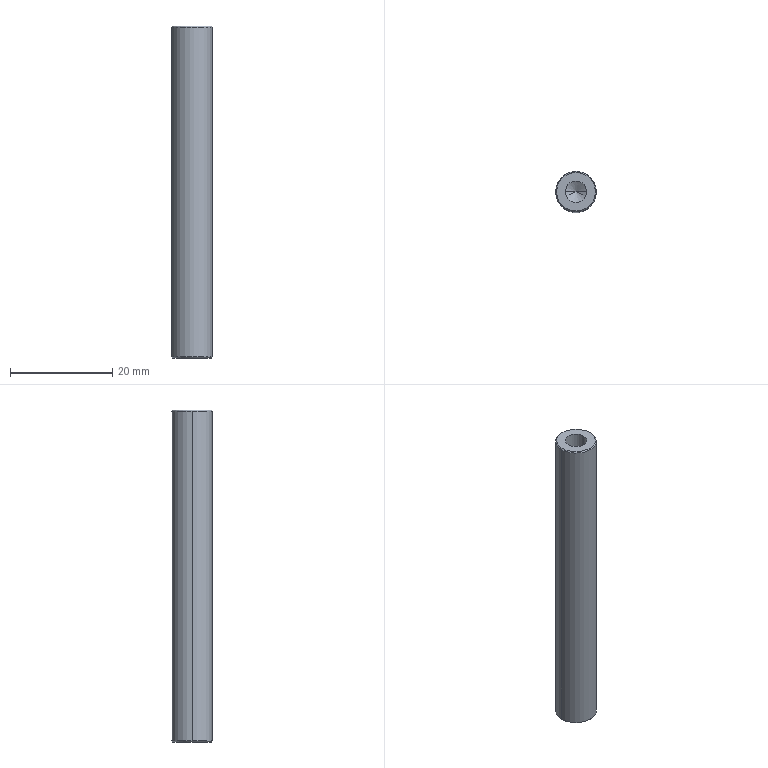Part | STEP file | 1 solid | 16 faces | box 8 x 8 x 65 mm | volume 2978 mm3 | cone 8 | cylinder 6 | plane 2 | commonest cylinder face diameters 4.2 x4 8 x2
STEP:
#1=CARTESIAN_POINT('',(0.,0.,0.));
#2=DIRECTION('',(0.,0.,1.));
#3=DIRECTION('',(1.,0.,0.));
#4=AXIS2_PLACEMENT_3D('',#1,#2,#3);
#5=CARTESIAN_POINT('',(-2.1,0.,-22.5));
#6=VERTEX_POINT('',#5);
#7=CARTESIAN_POINT('',(-2.1,0.,-32.5));
#8=VERTEX_POINT('',#7);
#9=CARTESIAN_POINT('',(-2.1,0.,-32.5));
#10=DIRECTION('',(0.,0.,-1.));
#11=VECTOR('',#10,1.);
#12=LINE('',#9,#11);
#13=CARTESIAN_POINT('',(0.,0.,-32.5));
#14=DIRECTION('',(0.,0.,-1.));
#15=DIRECTION('',(-1.,0.,0.));
#16=AXIS2_PLACEMENT_3D('',#13,#14,#15);
#17=CYLINDRICAL_SURFACE('',#16,2.1);
#18=CARTESIAN_POINT('',(6.283,0.));
#19=DIRECTION('',(0.,1.));
#20=VECTOR('',#19,1.);
#21=LINE('',#18,#20);
#22=(GEOMETRIC_REPRESENTATION_CONTEXT(2)PARAMETRIC_REPRESENTATION_CONTEXT()REPRESENTATION_CONTEXT('',''));
#23=DEFINITIONAL_REPRESENTATION('',(#21),#22);
#24=PCURVE('',#17,#23);
#25=CARTESIAN_POINT('',(0.,0.,-32.5));
#26=DIRECTION('',(0.,0.,-1.));
#27=DIRECTION('',(-1.,0.,0.));
#28=AXIS2_PLACEMENT_3D('',#25,#26,#27);
#29=CYLINDRICAL_SURFACE('',#28,2.1);
#30=CARTESIAN_POINT('',(0.,0.));
#31=DIRECTION('',(0.,1.));
#32=VECTOR('',#31,1.);
#33=LINE('',#30,#32);
#34=(GEOMETRIC_REPRESENTATION_CONTEXT(2)PARAMETRIC_REPRESENTATION_CONTEXT()REPRESENTATION_CONTEXT('',''));
#35=DEFINITIONAL_REPRESENTATION('',(#33),#34);
#36=PCURVE('',#29,#35);
#37=SURFACE_CURVE('',#12,(#24,#36),.PCURVE_S1.);
#38=EDGE_CURVE('',#6,#8,#37,.T.);
#39=ORIENTED_EDGE('',*,*,#38,.T.);
#40=CARTESIAN_POINT('',(2.1,0.,-32.5));
#41=VERTEX_POINT('',#40);
#42=CARTESIAN_POINT('',(0.,0.,-32.5));
#43=DIRECTION('',(0.,0.,-1.));
#44=DIRECTION('',(-1.,0.,0.));
#45=AXIS2_PLACEMENT_3D('',#42,#43,#44);
#46=CIRCLE('',#45,2.1);
#47=CARTESIAN_POINT('',(0.,0.));
#48=DIRECTION('',(1.,0.));
#49=VECTOR('',#48,1.);
#50=LINE('',#47,#49);
#51=(GEOMETRIC_REPRESENTATION_CONTEXT(2)PARAMETRIC_REPRESENTATION_CONTEXT()REPRESENTATION_CONTEXT('',''));
#52=DEFINITIONAL_REPRESENTATION('',(#50),#51);
#53=PCURVE('',#17,#52);
#54=CARTESIAN_POINT('',(0.,0.,-32.5));
#55=DIRECTION('',(0.,0.,1.));
#56=DIRECTION('',(1.,0.,0.));
#57=AXIS2_PLACEMENT_3D('',#54,#55,#56);
#58=PLANE('',#57);
#59=CARTESIAN_POINT('',(-2.1,0.));
#60=CARTESIAN_POINT('',(-2.1,3.637));
#61=CARTESIAN_POINT('',(1.05,1.819));
#62=CARTESIAN_POINT('',(4.2,0.));
#63=CARTESIAN_POINT('',(1.05,-1.819));
#64=CARTESIAN_POINT('',(-2.1,-3.637));
#65=CARTESIAN_POINT('',(-2.1,0.));
#66=(BOUNDED_CURVE()B_SPLINE_CURVE(2,(#59,#60,#61,#62,#63,#64,#65),.UNSPECIFIED.,.T.,.F.)B_SPLINE_CURVE_WITH_KNOTS((1,2,2,2,2,1),(-2.094,0.,2.094,4.189,6.283,8.378),.UNSPECIFIED.)CURVE()GEOMETRIC_REPRESENTATION_ITEM()RATIONAL_B_SPLINE_CURVE((1.,0.5,1.,0.5,1.,0.5,1.))REPRESENTATION_ITEM(''));
#67=(GEOMETRIC_REPRESENTATION_CONTEXT(2)PARAMETRIC_REPRESENTATION_CONTEXT()REPRESENTATION_CONTEXT('',''));
#68=DEFINITIONAL_REPRESENTATION('',(#66),#67);
#69=PCURVE('',#58,#68);
#70=SURFACE_CURVE('',#46,(#53,#69),.PCURVE_S1.);
#71=EDGE_CURVE('',#41,#8,#70,.T.);
#72=ORIENTED_EDGE('',*,*,#71,.F.);
#73=CARTESIAN_POINT('',(2.1,0.,-22.5));
#74=VERTEX_POINT('',#73);
#75=CARTESIAN_POINT('',(2.1,0.,-32.5));
#76=DIRECTION('',(0.,0.,-1.));
#77=VECTOR('',#76,1.);
#78=LINE('',#75,#77);
#79=CARTESIAN_POINT('',(3.142,0.));
#80=DIRECTION('',(0.,1.));
#81=VECTOR('',#80,1.);
#82=LINE('',#79,#81);
#83=(GEOMETRIC_REPRESENTATION_CONTEXT(2)PARAMETRIC_REPRESENTATION_CONTEXT()REPRESENTATION_CONTEXT('',''));
#84=DEFINITIONAL_REPRESENTATION('',(#82),#83);
#85=PCURVE('',#17,#84);
#86=CARTESIAN_POINT('',(3.142,0.));
#87=DIRECTION('',(0.,1.));
#88=VECTOR('',#87,1.);
#89=LINE('',#86,#88);
#90=(GEOMETRIC_REPRESENTATION_CONTEXT(2)PARAMETRIC_REPRESENTATION_CONTEXT()REPRESENTATION_CONTEXT('',''));
#91=DEFINITIONAL_REPRESENTATION('',(#89),#90);
#92=PCURVE('',#29,#91);
#93=SURFACE_CURVE('',#78,(#85,#92),.PCURVE_S1.);
#94=EDGE_CURVE('',#74,#41,#93,.T.);
#95=ORIENTED_EDGE('',*,*,#94,.F.);
#96=CARTESIAN_POINT('',(0.,0.,-22.5));
#97=DIRECTION('',(0.,0.,-1.));
#98=DIRECTION('',(-1.,0.,0.));
#99=AXIS2_PLACEMENT_3D('',#96,#97,#98);
#100=CIRCLE('',#99,2.1);
#101=CARTESIAN_POINT('',(0.,-10.));
#102=DIRECTION('',(1.,0.));
#103=VECTOR('',#102,1.);
#104=LINE('',#101,#103);
#105=(GEOMETRIC_REPRESENTATION_CONTEXT(2)PARAMETRIC_REPRESENTATION_CONTEXT()REPRESENTATION_CONTEXT('',''));
#106=DEFINITIONAL_REPRESENTATION('',(#104),#105);
#107=PCURVE('',#17,#106);
#108=CARTESIAN_POINT('',(0.,0.,-22.5));
#109=DIRECTION('',(0.,0.,-1.));
#110=DIRECTION('',(-1.,0.,0.));
#111=AXIS2_PLACEMENT_3D('',#108,#109,#110);
#112=CONICAL_SURFACE('',#111,2.1,1.03);
#113=CARTESIAN_POINT('',(0.,0.));
#114=DIRECTION('',(1.,0.));
#115=VECTOR('',#114,1.);
#116=LINE('',#113,#115);
#117=(GEOMETRIC_REPRESENTATION_CONTEXT(2)PARAMETRIC_REPRESENTATION_CONTEXT()REPRESENTATION_CONTEXT('',''));
#118=DEFINITIONAL_REPRESENTATION('',(#116),#117);
#119=PCURVE('',#112,#118);
#120=SURFACE_CURVE('',#100,(#107,#119),.PCURVE_S1.);
#121=EDGE_CURVE('',#74,#6,#120,.T.);
#122=ORIENTED_EDGE('',*,*,#121,.T.);
#123=EDGE_LOOP('',(#39,#72,#95,#122));
#124=FACE_BOUND('',#123,.F.);
#125=ADVANCED_FACE('',(#124),#17,.F.);
#126=ORIENTED_EDGE('',*,*,#121,.F.);
#127=CARTESIAN_POINT('',(0.,0.,-21.238));
#128=VERTEX_POINT('',#127);
#129=CARTESIAN_POINT('',(2.1,0.,-22.5));
#130=DIRECTION('',(0.8572,0.,-0.515));
#131=VECTOR('',#130,1.);
#132=LINE('',#129,#131);
#133=CARTESIAN_POINT('',(3.142,-1.262));
#134=CARTESIAN_POINT('',(3.142,-1.243));
#135=CARTESIAN_POINT('',(3.142,-1.204));
#136=CARTESIAN_POINT('',(3.142,-1.147));
#137=CARTESIAN_POINT('',(3.142,-1.09));
#138=CARTESIAN_POINT('',(3.142,-1.032));
#139=CARTESIAN_POINT('',(3.142,-0.975));
#140=CARTESIAN_POINT('',(3.142,-0.9177));
#141=CARTESIAN_POINT('',(3.142,-0.8603));
#142=CARTESIAN_POINT('',(3.142,-0.803));
#143=CARTESIAN_POINT('',(3.142,-0.7456));
#144=CARTESIAN_POINT('',(3.142,-0.6883));
#145=CARTESIAN_POINT('',(3.142,-0.6309));
#146=CARTESIAN_POINT('',(3.142,-0.5735));
#147=CARTESIAN_POINT('',(3.142,-0.5162));
#148=CARTESIAN_POINT('',(3.142,-0.4588));
#149=CARTESIAN_POINT('',(3.142,-0.4015));
#150=CARTESIAN_POINT('',(3.142,-0.3441));
#151=CARTESIAN_POINT('',(3.142,-0.2868));
#152=CARTESIAN_POINT('',(3.142,-0.2294));
#153=CARTESIAN_POINT('',(3.142,-0.1721));
#154=CARTESIAN_POINT('',(3.142,-0.1147));
#155=CARTESIAN_POINT('',(3.142,-0.05735));
#156=CARTESIAN_POINT('',(3.142,-0.01912));
#157=CARTESIAN_POINT('',(3.142,0.));
#158=B_SPLINE_CURVE_WITH_KNOTS('',3,(#133,#134,#135,#136,#137,#138,#139,#140,#141,#142,#143,#144,#145,#146,#147,#148,#149,#150,#151,#152,#153,#154,#155,#156,#157),.UNSPECIFIED.,.F.,.F.,(4,1,1,1,1,1,1,1,1,1,1,1,1,1,1,1,1,1,1,1,1,1,4),(-2.45,-2.339,-2.227,-2.116,-2.004,-1.893,-1.782,-1.67,-1.559,-1.448,-1.336,-1.225,-1.114,-1.002,-0.8909,-0.7795,-0.6682,-0.5568,-0.4454,-0.3341,-0.2227,-0.1114,0.),.QUASI_UNIFORM_KNOTS.);
#159=(GEOMETRIC_REPRESENTATION_CONTEXT(2)PARAMETRIC_REPRESENTATION_CONTEXT()REPRESENTATION_CONTEXT('',''));
#160=DEFINITIONAL_REPRESENTATION('',(#158),#159);
#161=PCURVE('',#112,#160);
#162=CARTESIAN_POINT('',(0.,0.,-22.5));
#163=DIRECTION('',(0.,0.,-1.));
#164=DIRECTION('',(-1.,0.,0.));
#165=AXIS2_PLACEMENT_3D('',#162,#163,#164);
#166=CONICAL_SURFACE('',#165,2.1,1.03);
#167=CARTESIAN_POINT('',(3.142,-1.262));
#168=CARTESIAN_POINT('',(3.142,-1.243));
#169=CARTESIAN_POINT('',(3.142,-1.204));
#170=CARTESIAN_POINT('',(3.142,-1.147));
#171=CARTESIAN_POINT('',(3.142,-1.09));
#172=CARTESIAN_POINT('',(3.142,-1.032));
#173=CARTESIAN_POINT('',(3.142,-0.975));
#174=CARTESIAN_POINT('',(3.142,-0.9177));
#175=CARTESIAN_POINT('',(3.142,-0.8603));
#176=CARTESIAN_POINT('',(3.142,-0.803));
#177=CARTESIAN_POINT('',(3.142,-0.7456));
#178=CARTESIAN_POINT('',(3.142,-0.6883));
#179=CARTESIAN_POINT('',(3.142,-0.6309));
#180=CARTESIAN_POINT('',(3.142,-0.5735));
#181=CARTESIAN_POINT('',(3.142,-0.5162));
#182=CARTESIAN_POINT('',(3.142,-0.4588));
#183=CARTESIAN_POINT('',(3.142,-0.4015));
#184=CARTESIAN_POINT('',(3.142,-0.3441));
#185=CARTESIAN_POINT('',(3.142,-0.2868));
#186=CARTESIAN_POINT('',(3.142,-0.2294));
#187=CARTESIAN_POINT('',(3.142,-0.1721));
#188=CARTESIAN_POINT('',(3.142,-0.1147));
#189=CARTESIAN_POINT('',(3.142,-0.05735));
#190=CARTESIAN_POINT('',(3.142,-0.01912));
#191=CARTESIAN_POINT('',(3.142,0.));
#192=B_SPLINE_CURVE_WITH_KNOTS('',3,(#167,#168,#169,#170,#171,#172,#173,#174,#175,#176,#177,#178,#179,#180,#181,#182,#183,#184,#185,#186,#187,#188,#189,#190,#191),.UNSPECIFIED.,.F.,.F.,(4,1,1,1,1,1,1,1,1,1,1,1,1,1,1,1,1,1,1,1,1,1,4),(-2.45,-2.339,-2.227,-2.116,-2.004,-1.893,-1.782,-1.67,-1.559,-1.448,-1.336,-1.225,-1.114,-1.002,-0.8909,-0.7795,-0.6682,-0.5568,-0.4454,-0.3341,-0.2227,-0.1114,0.),.QUASI_UNIFORM_KNOTS.);
#193=(GEOMETRIC_REPRESENTATION_CONTEXT(2)PARAMETRIC_REPRESENTATION_CONTEXT()REPRESENTATION_CONTEXT('',''));
#194=DEFINITIONAL_REPRESENTATION('',(#192),#193);
#195=PCURVE('',#166,#194);
#196=SURFACE_CURVE('',#132,(#161,#195),.PCURVE_S1.);
#197=EDGE_CURVE('',#128,#74,#196,.T.);
#198=ORIENTED_EDGE('',*,*,#197,.F.);
#199=CARTESIAN_POINT('',(-2.1,0.,-22.5));
#200=DIRECTION('',(-0.8572,0.,-0.515));
#201=VECTOR('',#200,1.);
#202=LINE('',#199,#201);
#203=CARTESIAN_POINT('',(6.283,0.));
#204=DIRECTION('',(0.,1.));
#205=VECTOR('',#204,1.);
#206=LINE('',#203,#205);
#207=(GEOMETRIC_REPRESENTATION_CONTEXT(2)PARAMETRIC_REPRESENTATION_CONTEXT()REPRESENTATION_CONTEXT('',''));
#208=DEFINITIONAL_REPRESENTATION('',(#206),#207);
#209=PCURVE('',#112,#208);
#210=CARTESIAN_POINT('',(0.,0.));
#211=DIRECTION('',(0.,1.));
#212=VECTOR('',#211,1.);
#213=LINE('',#210,#212);
#214=(GEOMETRIC_REPRESENTATION_CONTEXT(2)PARAMETRIC_REPRESENTATION_CONTEXT()REPRESENTATION_CONTEXT('',''));
#215=DEFINITIONAL_REPRESENTATION('',(#213),#214);
#216=PCURVE('',#166,#215);
#217=SURFACE_CURVE('',#202,(#209,#216),.PCURVE_S1.);
#218=EDGE_CURVE('',#128,#6,#217,.T.);
#219=ORIENTED_EDGE('',*,*,#218,.T.);
#220=EDGE_LOOP('',(#126,#198,#219));
#221=FACE_BOUND('',#220,.F.);
#222=ADVANCED_FACE('',(#221),#112,.F.);
#223=CARTESIAN_POINT('',(2.1,0.,22.5));
#224=VERTEX_POINT('',#223);
#225=CARTESIAN_POINT('',(2.1,0.,32.5));
#226=VERTEX_POINT('',#225);
#227=CARTESIAN_POINT('',(2.1,0.,32.5));
#228=DIRECTION('',(0.,0.,1.));
#229=VECTOR('',#228,1.);
#230=LINE('',#227,#229);
#231=CARTESIAN_POINT('',(0.,0.,32.5));
#232=DIRECTION('',(0.,0.,1.));
#233=DIRECTION('',(1.,0.,0.));
#234=AXIS2_PLACEMENT_3D('',#231,#232,#233);
#235=CYLINDRICAL_SURFACE('',#234,2.1);
#236=CARTESIAN_POINT('',(6.283,0.));
#237=DIRECTION('',(0.,1.));
#238=VECTOR('',#237,1.);
#239=LINE('',#236,#238);
#240=(GEOMETRIC_REPRESENTATION_CONTEXT(2)PARAMETRIC_REPRESENTATION_CONTEXT()REPRESENTATION_CONTEXT('',''));
#241=DEFINITIONAL_REPRESENTATION('',(#239),#240);
#242=PCURVE('',#235,#241);
#243=CARTESIAN_POINT('',(0.,0.,32.5));
#244=DIRECTION('',(0.,0.,1.));
#245=DIRECTION('',(1.,0.,0.));
#246=AXIS2_PLACEMENT_3D('',#243,#244,#245);
#247=CYLINDRICAL_SURFACE('',#246,2.1);
#248=CARTESIAN_POINT('',(0.,0.));
#249=DIRECTION('',(0.,1.));
#250=VECTOR('',#249,1.);
#251=LINE('',#248,#250);
#252=(GEOMETRIC_REPRESENTATION_CONTEXT(2)PARAMETRIC_REPRESENTATION_CONTEXT()REPRESENTATION_CONTEXT('',''));
#253=DEFINITIONAL_REPRESENTATION('',(#251),#252);
#254=PCURVE('',#247,#253);
#255=SURFACE_CURVE('',#230,(#242,#254),.PCURVE_S1.);
#256=EDGE_CURVE('',#224,#226,#255,.T.);
#257=ORIENTED_EDGE('',*,*,#256,.T.);
#258=CARTESIAN_POINT('',(-2.1,0.,32.5));
#259=VERTEX_POINT('',#258);
#260=CARTESIAN_POINT('',(0.,0.,32.5));
#261=DIRECTION('',(0.,0.,1.));
#262=DIRECTION('',(1.,0.,0.));
#263=AXIS2_PLACEMENT_3D('',#260,#261,#262);
#264=CIRCLE('',#263,2.1);
#265=CARTESIAN_POINT('',(0.,0.));
#266=DIRECTION('',(1.,0.));
#267=VECTOR('',#266,1.);
#268=LINE('',#265,#267);
#269=(GEOMETRIC_REPRESENTATION_CONTEXT(2)PARAMETRIC_REPRESENTATION_CONTEXT()REPRESENTATION_CONTEXT('',''));
#270=DEFINITIONAL_REPRESENTATION('',(#268),#269);
#271=PCURVE('',#235,#270);
#272=CARTESIAN_POINT('',(0.,0.,32.5));
#273=DIRECTION('',(0.,0.,1.));
#274=DIRECTION('',(1.,0.,0.));
#275=AXIS2_PLACEMENT_3D('',#272,#273,#274);
#276=PLANE('',#275);
#277=CARTESIAN_POINT('',(0.,0.));
#278=DIRECTION('',(1.,0.));
#279=AXIS2_PLACEMENT_2D('',#277,#278);
#280=CIRCLE('',#279,2.1);
#281=(GEOMETRIC_REPRESENTATION_CONTEXT(2)PARAMETRIC_REPRESENTATION_CONTEXT()REPRESENTATION_CONTEXT('',''));
#282=DEFINITIONAL_REPRESENTATION('',(#280),#281);
#283=PCURVE('',#276,#282);
#284=SURFACE_CURVE('',#264,(#271,#283),.PCURVE_S1.);
#285=EDGE_CURVE('',#259,#226,#284,.T.);
#286=ORIENTED_EDGE('',*,*,#285,.F.);
#287=CARTESIAN_POINT('',(-2.1,0.,22.5));
#288=VERTEX_POINT('',#287);
#289=CARTESIAN_POINT('',(-2.1,0.,32.5));
#290=DIRECTION('',(0.,0.,1.));
#291=VECTOR('',#290,1.);
#292=LINE('',#289,#291);
#293=CARTESIAN_POINT('',(3.142,0.));
#294=DIRECTION('',(0.,1.));
#295=VECTOR('',#294,1.);
#296=LINE('',#293,#295);
#297=(GEOMETRIC_REPRESENTATION_CONTEXT(2)PARAMETRIC_REPRESENTATION_CONTEXT()REPRESENTATION_CONTEXT('',''));
#298=DEFINITIONAL_REPRESENTATION('',(#296),#297);
#299=PCURVE('',#235,#298);
#300=CARTESIAN_POINT('',(3.142,0.));
#301=DIRECTION('',(0.,1.));
#302=VECTOR('',#301,1.);
#303=LINE('',#300,#302);
#304=(GEOMETRIC_REPRESENTATION_CONTEXT(2)PARAMETRIC_REPRESENTATION_CONTEXT()REPRESENTATION_CONTEXT('',''));
#305=DEFINITIONAL_REPRESENTATION('',(#303),#304);
#306=PCURVE('',#247,#305);
#307=SURFACE_CURVE('',#292,(#299,#306),.PCURVE_S1.);
#308=EDGE_CURVE('',#288,#259,#307,.T.);
#309=ORIENTED_EDGE('',*,*,#308,.F.);
#310=CARTESIAN_POINT('',(0.,0.,22.5));
#311=DIRECTION('',(0.,0.,1.));
#312=DIRECTION('',(1.,0.,0.));
#313=AXIS2_PLACEMENT_3D('',#310,#311,#312);
#314=CIRCLE('',#313,2.1);
#315=CARTESIAN_POINT('',(0.,-10.));
#316=DIRECTION('',(1.,0.));
#317=VECTOR('',#316,1.);
#318=LINE('',#315,#317);
#319=(GEOMETRIC_REPRESENTATION_CONTEXT(2)PARAMETRIC_REPRESENTATION_CONTEXT()REPRESENTATION_CONTEXT('',''));
#320=DEFINITIONAL_REPRESENTATION('',(#318),#319);
#321=PCURVE('',#235,#320);
#322=CARTESIAN_POINT('',(0.,0.,22.5));
#323=DIRECTION('',(0.,0.,1.));
#324=DIRECTION('',(1.,0.,0.));
#325=AXIS2_PLACEMENT_3D('',#322,#323,#324);
#326=CONICAL_SURFACE('',#325,2.1,1.03);
#327=CARTESIAN_POINT('',(0.,0.));
#328=DIRECTION('',(1.,0.));
#329=VECTOR('',#328,1.);
#330=LINE('',#327,#329);
#331=(GEOMETRIC_REPRESENTATION_CONTEXT(2)PARAMETRIC_REPRESENTATION_CONTEXT()REPRESENTATION_CONTEXT('',''));
#332=DEFINITIONAL_REPRESENTATION('',(#330),#331);
#333=PCURVE('',#326,#332);
#334=SURFACE_CURVE('',#314,(#321,#333),.PCURVE_S1.);
#335=EDGE_CURVE('',#288,#224,#334,.T.);
#336=ORIENTED_EDGE('',*,*,#335,.T.);
#337=EDGE_LOOP('',(#257,#286,#309,#336));
#338=FACE_BOUND('',#337,.F.);
#339=ADVANCED_FACE('',(#338),#235,.F.);
#340=ORIENTED_EDGE('',*,*,#335,.F.);
#341=CARTESIAN_POINT('',(0.,0.,21.238));
#342=VERTEX_POINT('',#341);
#343=CARTESIAN_POINT('',(-2.1,0.,22.5));
#344=DIRECTION('',(-0.8572,0.,0.515));
#345=VECTOR('',#344,1.);
#346=LINE('',#343,#345);
#347=CARTESIAN_POINT('',(3.142,0.));
#348=DIRECTION('',(0.,1.));
#349=VECTOR('',#348,1.);
#350=LINE('',#347,#349);
#351=(GEOMETRIC_REPRESENTATION_CONTEXT(2)PARAMETRIC_REPRESENTATION_CONTEXT()REPRESENTATION_CONTEXT('',''));
#352=DEFINITIONAL_REPRESENTATION('',(#350),#351);
#353=PCURVE('',#326,#352);
#354=CARTESIAN_POINT('',(0.,0.,22.5));
#355=DIRECTION('',(0.,0.,1.));
#356=DIRECTION('',(1.,0.,0.));
#357=AXIS2_PLACEMENT_3D('',#354,#355,#356);
#358=CONICAL_SURFACE('',#357,2.1,1.03);
#359=CARTESIAN_POINT('',(3.142,0.));
#360=DIRECTION('',(0.,1.));
#361=VECTOR('',#360,1.);
#362=LINE('',#359,#361);
#363=(GEOMETRIC_REPRESENTATION_CONTEXT(2)PARAMETRIC_REPRESENTATION_CONTEXT()REPRESENTATION_CONTEXT('',''));
#364=DEFINITIONAL_REPRESENTATION('',(#362),#363);
#365=PCURVE('',#358,#364);
#366=SURFACE_CURVE('',#346,(#353,#365),.PCURVE_S1.);
#367=EDGE_CURVE('',#342,#288,#366,.T.);
#368=ORIENTED_EDGE('',*,*,#367,.F.);
#369=CARTESIAN_POINT('',(2.1,0.,22.5));
#370=DIRECTION('',(0.8572,0.,0.515));
#371=VECTOR('',#370,1.);
#372=LINE('',#369,#371);
#373=CARTESIAN_POINT('',(6.283,-1.262));
#374=CARTESIAN_POINT('',(6.283,-1.243));
#375=CARTESIAN_POINT('',(6.283,-1.204));
#376=CARTESIAN_POINT('',(6.283,-1.147));
#377=CARTESIAN_POINT('',(6.283,-1.09));
#378=CARTESIAN_POINT('',(6.283,-1.032));
#379=CARTESIAN_POINT('',(6.283,-0.975));
#380=CARTESIAN_POINT('',(6.283,-0.9177));
#381=CARTESIAN_POINT('',(6.283,-0.8603));
#382=CARTESIAN_POINT('',(6.283,-0.803));
#383=CARTESIAN_POINT('',(6.283,-0.7456));
#384=CARTESIAN_POINT('',(6.283,-0.6883));
#385=CARTESIAN_POINT('',(6.283,-0.6309));
#386=CARTESIAN_POINT('',(6.283,-0.5735));
#387=CARTESIAN_POINT('',(6.283,-0.5162));
#388=CARTESIAN_POINT('',(6.283,-0.4588));
#389=CARTESIAN_POINT('',(6.283,-0.4015));
#390=CARTESIAN_POINT('',(6.283,-0.3441));
#391=CARTESIAN_POINT('',(6.283,-0.2868));
#392=CARTESIAN_POINT('',(6.283,-0.2294));
#393=CARTESIAN_POINT('',(6.283,-0.1721));
#394=CARTESIAN_POINT('',(6.283,-0.1147));
#395=CARTESIAN_POINT('',(6.283,-0.05735));
#396=CARTESIAN_POINT('',(6.283,-0.01912));
#397=CARTESIAN_POINT('',(6.283,0.));
#398=B_SPLINE_CURVE_WITH_KNOTS('',3,(#373,#374,#375,#376,#377,#378,#379,#380,#381,#382,#383,#384,#385,#386,#387,#388,#389,#390,#391,#392,#393,#394,#395,#396,#397),.UNSPECIFIED.,.F.,.F.,(4,1,1,1,1,1,1,1,1,1,1,1,1,1,1,1,1,1,1,1,1,1,4),(-2.45,-2.339,-2.227,-2.116,-2.004,-1.893,-1.782,-1.67,-1.559,-1.448,-1.336,-1.225,-1.114,-1.002,-0.8909,-0.7795,-0.6682,-0.5568,-0.4454,-0.3341,-0.2227,-0.1114,0.),.QUASI_UNIFORM_KNOTS.);
#399=(GEOMETRIC_REPRESENTATION_CONTEXT(2)PARAMETRIC_REPRESENTATION_CONTEXT()REPRESENTATION_CONTEXT('',''));
#400=DEFINITIONAL_REPRESENTATION('',(#398),#399);
#401=PCURVE('',#326,#400);
#402=CARTESIAN_POINT('',(0.,-1.262));
#403=CARTESIAN_POINT('',(0.,-1.243));
#404=CARTESIAN_POINT('',(0.,-1.204));
#405=CARTESIAN_POINT('',(0.,-1.147));
#406=CARTESIAN_POINT('',(0.,-1.09));
#407=CARTESIAN_POINT('',(0.,-1.032));
#408=CARTESIAN_POINT('',(0.,-0.975));
#409=CARTESIAN_POINT('',(0.,-0.9177));
#410=CARTESIAN_POINT('',(0.,-0.8603));
#411=CARTESIAN_POINT('',(0.,-0.803));
#412=CARTESIAN_POINT('',(0.,-0.7456));
#413=CARTESIAN_POINT('',(0.,-0.6883));
#414=CARTESIAN_POINT('',(0.,-0.6309));
#415=CARTESIAN_POINT('',(0.,-0.5735));
#416=CARTESIAN_POINT('',(0.,-0.5162));
#417=CARTESIAN_POINT('',(0.,-0.4588));
#418=CARTESIAN_POINT('',(0.,-0.4015));
#419=CARTESIAN_POINT('',(0.,-0.3441));
#420=CARTESIAN_POINT('',(0.,-0.2868));
#421=CARTESIAN_POINT('',(0.,-0.2294));
#422=CARTESIAN_POINT('',(0.,-0.1721));
#423=CARTESIAN_POINT('',(0.,-0.1147));
#424=CARTESIAN_POINT('',(0.,-0.05735));
#425=CARTESIAN_POINT('',(0.,-0.01912));
#426=CARTESIAN_POINT('',(0.,0.));
#427=B_SPLINE_CURVE_WITH_KNOTS('',3,(#402,#403,#404,#405,#406,#407,#408,#409,#410,#411,#412,#413,#414,#415,#416,#417,#418,#419,#420,#421,#422,#423,#424,#425,#426),.UNSPECIFIED.,.F.,.F.,(4,1,1,1,1,1,1,1,1,1,1,1,1,1,1,1,1,1,1,1,1,1,4),(-2.45,-2.339,-2.227,-2.116,-2.004,-1.893,-1.782,-1.67,-1.559,-1.448,-1.336,-1.225,-1.114,-1.002,-0.8909,-0.7795,-0.6682,-0.5568,-0.4454,-0.3341,-0.2227,-0.1114,0.),.QUASI_UNIFORM_KNOTS.);
#428=(GEOMETRIC_REPRESENTATION_CONTEXT(2)PARAMETRIC_REPRESENTATION_CONTEXT()REPRESENTATION_CONTEXT('',''));
#429=DEFINITIONAL_REPRESENTATION('',(#427),#428);
#430=PCURVE('',#358,#429);
#431=SURFACE_CURVE('',#372,(#401,#430),.PCURVE_S1.);
#432=EDGE_CURVE('',#342,#224,#431,.T.);
#433=ORIENTED_EDGE('',*,*,#432,.T.);
#434=EDGE_LOOP('',(#340,#368,#433));
#435=FACE_BOUND('',#434,.F.);
#436=ADVANCED_FACE('',(#435),#326,.F.);
#437=CARTESIAN_POINT('',(3.8,0.,32.5));
#438=VERTEX_POINT('',#437);
#439=CARTESIAN_POINT('',(-3.8,0.,32.5));
#440=VERTEX_POINT('',#439);
#441=CARTESIAN_POINT('',(0.,0.,32.5));
#442=DIRECTION('',(0.,0.,1.));
#443=DIRECTION('',(1.,0.,0.));
#444=AXIS2_PLACEMENT_3D('',#441,#442,#443);
#445=CIRCLE('',#444,3.8);
#446=CARTESIAN_POINT('',(0.,0.,32.5));
#447=DIRECTION('',(0.,0.,-1.));
#448=DIRECTION('',(-1.,0.,0.));
#449=AXIS2_PLACEMENT_3D('',#446,#447,#448);
#450=CONICAL_SURFACE('',#449,3.8,0.7854);
#451=CARTESIAN_POINT('',(3.142,0.));
#452=DIRECTION('',(-1.,0.));
#453=VECTOR('',#452,1.);
#454=LINE('',#451,#453);
#455=(GEOMETRIC_REPRESENTATION_CONTEXT(2)PARAMETRIC_REPRESENTATION_CONTEXT()REPRESENTATION_CONTEXT('',''));
#456=DEFINITIONAL_REPRESENTATION('',(#454),#455);
#457=PCURVE('',#450,#456);
#458=CARTESIAN_POINT('',(0.,0.));
#459=DIRECTION('',(1.,0.));
#460=AXIS2_PLACEMENT_2D('',#458,#459);
#461=CIRCLE('',#460,3.8);
#462=(GEOMETRIC_REPRESENTATION_CONTEXT(2)PARAMETRIC_REPRESENTATION_CONTEXT()REPRESENTATION_CONTEXT('',''));
#463=DEFINITIONAL_REPRESENTATION('',(#461),#462);
#464=PCURVE('',#276,#463);
#465=SURFACE_CURVE('',#445,(#457,#464),.PCURVE_S1.);
#466=EDGE_CURVE('',#438,#440,#465,.T.);
#467=ORIENTED_EDGE('',*,*,#466,.F.);
#468=CARTESIAN_POINT('',(4.,0.,32.3));
#469=VERTEX_POINT('',#468);
#470=CARTESIAN_POINT('',(3.8,0.,32.5));
#471=DIRECTION('',(0.7071,0.,-0.7071));
#472=VECTOR('',#471,1.);
#473=LINE('',#470,#472);
#474=CARTESIAN_POINT('',(3.142,0.));
#475=DIRECTION('',(0.,1.));
#476=VECTOR('',#475,1.);
#477=LINE('',#474,#476);
#478=(GEOMETRIC_REPRESENTATION_CONTEXT(2)PARAMETRIC_REPRESENTATION_CONTEXT()REPRESENTATION_CONTEXT('',''));
#479=DEFINITIONAL_REPRESENTATION('',(#477),#478);
#480=PCURVE('',#450,#479);
#481=CARTESIAN_POINT('',(0.,0.,32.5));
#482=DIRECTION('',(0.,0.,-1.));
#483=DIRECTION('',(-1.,0.,0.));
#484=AXIS2_PLACEMENT_3D('',#481,#482,#483);
#485=CONICAL_SURFACE('',#484,3.8,0.7854);
#486=CARTESIAN_POINT('',(3.142,0.));
#487=DIRECTION('',(0.,1.));
#488=VECTOR('',#487,1.);
#489=LINE('',#486,#488);
#490=(GEOMETRIC_REPRESENTATION_CONTEXT(2)PARAMETRIC_REPRESENTATION_CONTEXT()REPRESENTATION_CONTEXT('',''));
#491=DEFINITIONAL_REPRESENTATION('',(#489),#490);
#492=PCURVE('',#485,#491);
#493=SURFACE_CURVE('',#473,(#480,#492),.PCURVE_S1.);
#494=EDGE_CURVE('',#438,#469,#493,.T.);
#495=ORIENTED_EDGE('',*,*,#494,.T.);
#496=CARTESIAN_POINT('',(-4.,0.,32.3));
#497=VERTEX_POINT('',#496);
#498=CARTESIAN_POINT('',(0.,0.,32.3));
#499=DIRECTION('',(0.,0.,-1.));
#500=DIRECTION('',(1.,0.,0.));
#501=AXIS2_PLACEMENT_3D('',#498,#499,#500);
#502=CIRCLE('',#501,4.);
#503=CARTESIAN_POINT('',(-3.142,0.2));
#504=DIRECTION('',(1.,0.));
#505=VECTOR('',#504,1.);
#506=LINE('',#503,#505);
#507=(GEOMETRIC_REPRESENTATION_CONTEXT(2)PARAMETRIC_REPRESENTATION_CONTEXT()REPRESENTATION_CONTEXT('',''));
#508=DEFINITIONAL_REPRESENTATION('',(#506),#507);
#509=PCURVE('',#450,#508);
#510=CARTESIAN_POINT('',(0.,0.,32.5));
#511=DIRECTION('',(0.,0.,-1.));
#512=DIRECTION('',(-1.,0.,0.));
#513=AXIS2_PLACEMENT_3D('',#510,#511,#512);
#514=CYLINDRICAL_SURFACE('',#513,4.);
#515=CARTESIAN_POINT('',(-3.142,0.2));
#516=DIRECTION('',(1.,0.));
#517=VECTOR('',#516,1.);
#518=LINE('',#515,#517);
#519=(GEOMETRIC_REPRESENTATION_CONTEXT(2)PARAMETRIC_REPRESENTATION_CONTEXT()REPRESENTATION_CONTEXT('',''));
#520=DEFINITIONAL_REPRESENTATION('',(#518),#519);
#521=PCURVE('',#514,#520);
#522=SURFACE_CURVE('',#502,(#509,#521),.PCURVE_S1.);
#523=EDGE_CURVE('',#497,#469,#522,.T.);
#524=ORIENTED_EDGE('',*,*,#523,.F.);
#525=CARTESIAN_POINT('',(-3.8,0.,32.5));
#526=DIRECTION('',(-0.7071,0.,-0.7071));
#527=VECTOR('',#526,1.);
#528=LINE('',#525,#527);
#529=CARTESIAN_POINT('',(0.,0.));
#530=DIRECTION('',(0.,1.));
#531=VECTOR('',#530,1.);
#532=LINE('',#529,#531);
#533=(GEOMETRIC_REPRESENTATION_CONTEXT(2)PARAMETRIC_REPRESENTATION_CONTEXT()REPRESENTATION_CONTEXT('',''));
#534=DEFINITIONAL_REPRESENTATION('',(#532),#533);
#535=PCURVE('',#450,#534);
#536=CARTESIAN_POINT('',(6.283,0.));
#537=DIRECTION('',(0.,1.));
#538=VECTOR('',#537,1.);
#539=LINE('',#536,#538);
#540=(GEOMETRIC_REPRESENTATION_CONTEXT(2)PARAMETRIC_REPRESENTATION_CONTEXT()REPRESENTATION_CONTEXT('',''));
#541=DEFINITIONAL_REPRESENTATION('',(#539),#540);
#542=PCURVE('',#485,#541);
#543=SURFACE_CURVE('',#528,(#535,#542),.PCURVE_S1.);
#544=EDGE_CURVE('',#440,#497,#543,.T.);
#545=ORIENTED_EDGE('',*,*,#544,.F.);
#546=EDGE_LOOP('',(#467,#495,#524,#545));
#547=FACE_BOUND('',#546,.T.);
#548=ADVANCED_FACE('',(#547),#450,.T.);
#549=CARTESIAN_POINT('',(-3.8,0.,-32.5));
#550=VERTEX_POINT('',#549);
#551=CARTESIAN_POINT('',(3.8,0.,-32.5));
#552=VERTEX_POINT('',#551);
#553=CARTESIAN_POINT('',(0.,0.,-32.5));
#554=DIRECTION('',(0.,0.,-1.));
#555=DIRECTION('',(1.,0.,0.));
#556=AXIS2_PLACEMENT_3D('',#553,#554,#555);
#557=CIRCLE('',#556,3.8);
#558=CARTESIAN_POINT('',(0.,0.,-32.3));
#559=DIRECTION('',(0.,0.,1.));
#560=DIRECTION('',(1.,0.,0.));
#561=AXIS2_PLACEMENT_3D('',#558,#559,#560);
#562=CONICAL_SURFACE('',#561,4.,0.7854);
#563=CARTESIAN_POINT('',(6.283,-0.2));
#564=DIRECTION('',(-1.,0.));
#565=VECTOR('',#564,1.);
#566=LINE('',#563,#565);
#567=(GEOMETRIC_REPRESENTATION_CONTEXT(2)PARAMETRIC_REPRESENTATION_CONTEXT()REPRESENTATION_CONTEXT('',''));
#568=DEFINITIONAL_REPRESENTATION('',(#566),#567);
#569=PCURVE('',#562,#568);
#570=CARTESIAN_POINT('',(3.8,0.));
#571=CARTESIAN_POINT('',(3.8,-6.582));
#572=CARTESIAN_POINT('',(-1.9,-3.291));
#573=CARTESIAN_POINT('',(-7.6,0.));
#574=CARTESIAN_POINT('',(-1.9,3.291));
#575=CARTESIAN_POINT('',(3.8,6.582));
#576=CARTESIAN_POINT('',(3.8,0.));
#577=(BOUNDED_CURVE()B_SPLINE_CURVE(2,(#570,#571,#572,#573,#574,#575,#576),.UNSPECIFIED.,.T.,.F.)B_SPLINE_CURVE_WITH_KNOTS((1,2,2,2,2,1),(-2.094,0.,2.094,4.189,6.283,8.378),.UNSPECIFIED.)CURVE()GEOMETRIC_REPRESENTATION_ITEM()RATIONAL_B_SPLINE_CURVE((1.,0.5,1.,0.5,1.,0.5,1.))REPRESENTATION_ITEM(''));
#578=(GEOMETRIC_REPRESENTATION_CONTEXT(2)PARAMETRIC_REPRESENTATION_CONTEXT()REPRESENTATION_CONTEXT('',''));
#579=DEFINITIONAL_REPRESENTATION('',(#577),#578);
#580=PCURVE('',#58,#579);
#581=SURFACE_CURVE('',#557,(#569,#580),.PCURVE_S1.);
#582=EDGE_CURVE('',#550,#552,#581,.T.);
#583=ORIENTED_EDGE('',*,*,#582,.F.);
#584=CARTESIAN_POINT('',(-4.,0.,-32.3));
#585=VERTEX_POINT('',#584);
#586=CARTESIAN_POINT('',(-4.,0.,-32.3));
#587=DIRECTION('',(-0.7071,0.,0.7071));
#588=VECTOR('',#587,1.);
#589=LINE('',#586,#588);
#590=CARTESIAN_POINT('',(3.142,0.));
#591=DIRECTION('',(0.,1.));
#592=VECTOR('',#591,1.);
#593=LINE('',#590,#592);
#594=(GEOMETRIC_REPRESENTATION_CONTEXT(2)PARAMETRIC_REPRESENTATION_CONTEXT()REPRESENTATION_CONTEXT('',''));
#595=DEFINITIONAL_REPRESENTATION('',(#593),#594);
#596=PCURVE('',#562,#595);
#597=CARTESIAN_POINT('',(0.,0.,-32.3));
#598=DIRECTION('',(0.,0.,1.));
#599=DIRECTION('',(1.,0.,0.));
#600=AXIS2_PLACEMENT_3D('',#597,#598,#599);
#601=CONICAL_SURFACE('',#600,4.,0.7854);
#602=CARTESIAN_POINT('',(3.142,0.));
#603=DIRECTION('',(0.,1.));
#604=VECTOR('',#603,1.);
#605=LINE('',#602,#604);
#606=(GEOMETRIC_REPRESENTATION_CONTEXT(2)PARAMETRIC_REPRESENTATION_CONTEXT()REPRESENTATION_CONTEXT('',''));
#607=DEFINITIONAL_REPRESENTATION('',(#605),#606);
#608=PCURVE('',#601,#607);
#609=SURFACE_CURVE('',#589,(#596,#608),.PCURVE_S1.);
#610=EDGE_CURVE('',#550,#585,#609,.T.);
#611=ORIENTED_EDGE('',*,*,#610,.T.);
#612=CARTESIAN_POINT('',(4.,0.,-32.3));
#613=VERTEX_POINT('',#612);
#614=CARTESIAN_POINT('',(0.,0.,-32.3));
#615=DIRECTION('',(0.,0.,1.));
#616=DIRECTION('',(1.,0.,0.));
#617=AXIS2_PLACEMENT_3D('',#614,#615,#616);
#618=CIRCLE('',#617,4.);
#619=CARTESIAN_POINT('',(0.,0.));
#620=DIRECTION('',(1.,0.));
#621=VECTOR('',#620,1.);
#622=LINE('',#619,#621);
#623=(GEOMETRIC_REPRESENTATION_CONTEXT(2)PARAMETRIC_REPRESENTATION_CONTEXT()REPRESENTATION_CONTEXT('',''));
#624=DEFINITIONAL_REPRESENTATION('',(#622),#623);
#625=PCURVE('',#562,#624);
#626=CARTESIAN_POINT('',(3.142,64.8));
#627=DIRECTION('',(-1.,0.));
#628=VECTOR('',#627,1.);
#629=LINE('',#626,#628);
#630=(GEOMETRIC_REPRESENTATION_CONTEXT(2)PARAMETRIC_REPRESENTATION_CONTEXT()REPRESENTATION_CONTEXT('',''));
#631=DEFINITIONAL_REPRESENTATION('',(#629),#630);
#632=PCURVE('',#514,#631);
#633=SURFACE_CURVE('',#618,(#625,#632),.PCURVE_S1.);
#634=EDGE_CURVE('',#613,#585,#633,.T.);
#635=ORIENTED_EDGE('',*,*,#634,.F.);
#636=CARTESIAN_POINT('',(4.,0.,-32.3));
#637=DIRECTION('',(0.7071,0.,0.7071));
#638=VECTOR('',#637,1.);
#639=LINE('',#636,#638);
#640=CARTESIAN_POINT('',(0.,0.));
#641=DIRECTION('',(0.,1.));
#642=VECTOR('',#641,1.);
#643=LINE('',#640,#642);
#644=(GEOMETRIC_REPRESENTATION_CONTEXT(2)PARAMETRIC_REPRESENTATION_CONTEXT()REPRESENTATION_CONTEXT('',''));
#645=DEFINITIONAL_REPRESENTATION('',(#643),#644);
#646=PCURVE('',#562,#645);
#647=CARTESIAN_POINT('',(6.283,0.));
#648=DIRECTION('',(0.,1.));
#649=VECTOR('',#648,1.);
#650=LINE('',#647,#649);
#651=(GEOMETRIC_REPRESENTATION_CONTEXT(2)PARAMETRIC_REPRESENTATION_CONTEXT()REPRESENTATION_CONTEXT('',''));
#652=DEFINITIONAL_REPRESENTATION('',(#650),#651);
#653=PCURVE('',#601,#652);
#654=SURFACE_CURVE('',#639,(#646,#653),.PCURVE_S1.);
#655=EDGE_CURVE('',#552,#613,#654,.T.);
#656=ORIENTED_EDGE('',*,*,#655,.F.);
#657=EDGE_LOOP('',(#583,#611,#635,#656));
#658=FACE_BOUND('',#657,.T.);
#659=ADVANCED_FACE('',(#658),#562,.T.);
#660=ORIENTED_EDGE('',*,*,#523,.T.);
#661=CARTESIAN_POINT('',(4.,0.,32.5));
#662=DIRECTION('',(0.,0.,-1.));
#663=VECTOR('',#662,1.);
#664=LINE('',#661,#663);
#665=CARTESIAN_POINT('',(3.142,0.));
#666=DIRECTION('',(0.,1.));
#667=VECTOR('',#666,1.);
#668=LINE('',#665,#667);
#669=(GEOMETRIC_REPRESENTATION_CONTEXT(2)PARAMETRIC_REPRESENTATION_CONTEXT()REPRESENTATION_CONTEXT('',''));
#670=DEFINITIONAL_REPRESENTATION('',(#668),#669);
#671=PCURVE('',#514,#670);
#672=CARTESIAN_POINT('',(0.,0.,32.5));
#673=DIRECTION('',(0.,0.,-1.));
#674=DIRECTION('',(-1.,0.,0.));
#675=AXIS2_PLACEMENT_3D('',#672,#673,#674);
#676=CYLINDRICAL_SURFACE('',#675,4.);
#677=CARTESIAN_POINT('',(3.142,0.));
#678=DIRECTION('',(0.,1.));
#679=VECTOR('',#678,1.);
#680=LINE('',#677,#679);
#681=(GEOMETRIC_REPRESENTATION_CONTEXT(2)PARAMETRIC_REPRESENTATION_CONTEXT()REPRESENTATION_CONTEXT('',''));
#682=DEFINITIONAL_REPRESENTATION('',(#680),#681);
#683=PCURVE('',#676,#682);
#684=SURFACE_CURVE('',#664,(#671,#683),.PCURVE_S1.);
#685=EDGE_CURVE('',#469,#613,#684,.T.);
#686=ORIENTED_EDGE('',*,*,#685,.T.);
#687=ORIENTED_EDGE('',*,*,#634,.T.);
#688=CARTESIAN_POINT('',(-4.,0.,32.5));
#689=DIRECTION('',(0.,0.,-1.));
#690=VECTOR('',#689,1.);
#691=LINE('',#688,#690);
#692=CARTESIAN_POINT('',(0.,0.));
#693=DIRECTION('',(0.,1.));
#694=VECTOR('',#693,1.);
#695=LINE('',#692,#694);
#696=(GEOMETRIC_REPRESENTATION_CONTEXT(2)PARAMETRIC_REPRESENTATION_CONTEXT()REPRESENTATION_CONTEXT('',''));
#697=DEFINITIONAL_REPRESENTATION('',(#695),#696);
#698=PCURVE('',#514,#697);
#699=CARTESIAN_POINT('',(6.283,0.));
#700=DIRECTION('',(0.,1.));
#701=VECTOR('',#700,1.);
#702=LINE('',#699,#701);
#703=(GEOMETRIC_REPRESENTATION_CONTEXT(2)PARAMETRIC_REPRESENTATION_CONTEXT()REPRESENTATION_CONTEXT('',''));
#704=DEFINITIONAL_REPRESENTATION('',(#702),#703);
#705=PCURVE('',#676,#704);
#706=SURFACE_CURVE('',#691,(#698,#705),.PCURVE_S1.);
#707=EDGE_CURVE('',#497,#585,#706,.T.);
#708=ORIENTED_EDGE('',*,*,#707,.F.);
#709=EDGE_LOOP('',(#660,#686,#687,#708));
#710=FACE_BOUND('',#709,.T.);
#711=ADVANCED_FACE('',(#710),#514,.T.);
#712=ORIENTED_EDGE('',*,*,#685,.F.);
#713=CARTESIAN_POINT('',(0.,0.,32.3));
#714=DIRECTION('',(0.,0.,-1.));
#715=DIRECTION('',(1.,0.,0.));
#716=AXIS2_PLACEMENT_3D('',#713,#714,#715);
#717=CIRCLE('',#716,4.);
#718=CARTESIAN_POINT('',(3.142,0.2));
#719=DIRECTION('',(1.,0.));
#720=VECTOR('',#719,1.);
#721=LINE('',#718,#720);
#722=(GEOMETRIC_REPRESENTATION_CONTEXT(2)PARAMETRIC_REPRESENTATION_CONTEXT()REPRESENTATION_CONTEXT('',''));
#723=DEFINITIONAL_REPRESENTATION('',(#721),#722);
#724=PCURVE('',#676,#723);
#725=CARTESIAN_POINT('',(3.142,0.2));
#726=DIRECTION('',(1.,0.));
#727=VECTOR('',#726,1.);
#728=LINE('',#725,#727);
#729=(GEOMETRIC_REPRESENTATION_CONTEXT(2)PARAMETRIC_REPRESENTATION_CONTEXT()REPRESENTATION_CONTEXT('',''));
#730=DEFINITIONAL_REPRESENTATION('',(#728),#729);
#731=PCURVE('',#485,#730);
#732=SURFACE_CURVE('',#717,(#724,#731),.PCURVE_S1.);
#733=EDGE_CURVE('',#469,#497,#732,.T.);
#734=ORIENTED_EDGE('',*,*,#733,.T.);
#735=ORIENTED_EDGE('',*,*,#707,.T.);
#736=CARTESIAN_POINT('',(0.,0.,-32.3));
#737=DIRECTION('',(0.,0.,1.));
#738=DIRECTION('',(1.,0.,0.));
#739=AXIS2_PLACEMENT_3D('',#736,#737,#738);
#740=CIRCLE('',#739,4.);
#741=CARTESIAN_POINT('',(9.425,64.8));
#742=DIRECTION('',(-1.,0.));
#743=VECTOR('',#742,1.);
#744=LINE('',#741,#743);
#745=(GEOMETRIC_REPRESENTATION_CONTEXT(2)PARAMETRIC_REPRESENTATION_CONTEXT()REPRESENTATION_CONTEXT('',''));
#746=DEFINITIONAL_REPRESENTATION('',(#744),#745);
#747=PCURVE('',#676,#746);
#748=CARTESIAN_POINT('',(0.,0.));
#749=DIRECTION('',(1.,0.));
#750=VECTOR('',#749,1.);
#751=LINE('',#748,#750);
#752=(GEOMETRIC_REPRESENTATION_CONTEXT(2)PARAMETRIC_REPRESENTATION_CONTEXT()REPRESENTATION_CONTEXT('',''));
#753=DEFINITIONAL_REPRESENTATION('',(#751),#752);
#754=PCURVE('',#601,#753);
#755=SURFACE_CURVE('',#740,(#747,#754),.PCURVE_S1.);
#756=EDGE_CURVE('',#585,#613,#755,.T.);
#757=ORIENTED_EDGE('',*,*,#756,.T.);
#758=EDGE_LOOP('',(#712,#734,#735,#757));
#759=FACE_BOUND('',#758,.T.);
#760=ADVANCED_FACE('',(#759),#676,.T.);
#761=CARTESIAN_POINT('',(0.,0.,32.5));
#762=DIRECTION('',(0.,0.,1.));
#763=DIRECTION('',(1.,0.,0.));
#764=AXIS2_PLACEMENT_3D('',#761,#762,#763);
#765=CIRCLE('',#764,2.1);
#766=CARTESIAN_POINT('',(0.,0.));
#767=DIRECTION('',(1.,0.));
#768=AXIS2_PLACEMENT_2D('',#766,#767);
#769=CIRCLE('',#768,2.1);
#770=(GEOMETRIC_REPRESENTATION_CONTEXT(2)PARAMETRIC_REPRESENTATION_CONTEXT()REPRESENTATION_CONTEXT('',''));
#771=DEFINITIONAL_REPRESENTATION('',(#769),#770);
#772=PCURVE('',#276,#771);
#773=CARTESIAN_POINT('',(0.,0.));
#774=DIRECTION('',(1.,0.));
#775=VECTOR('',#774,1.);
#776=LINE('',#773,#775);
#777=(GEOMETRIC_REPRESENTATION_CONTEXT(2)PARAMETRIC_REPRESENTATION_CONTEXT()REPRESENTATION_CONTEXT('',''));
#778=DEFINITIONAL_REPRESENTATION('',(#776),#777);
#779=PCURVE('',#247,#778);
#780=SURFACE_CURVE('',#765,(#772,#779),.PCURVE_S1.);
#781=EDGE_CURVE('',#226,#259,#780,.T.);
#782=ORIENTED_EDGE('',*,*,#781,.F.);
#783=ORIENTED_EDGE('',*,*,#285,.F.);
#784=EDGE_LOOP('',(#782,#783));
#785=FACE_BOUND('',#784,.T.);
#786=CARTESIAN_POINT('',(0.,0.,32.5));
#787=DIRECTION('',(0.,0.,1.));
#788=DIRECTION('',(1.,0.,0.));
#789=AXIS2_PLACEMENT_3D('',#786,#787,#788);
#790=CIRCLE('',#789,3.8);
#791=CARTESIAN_POINT('',(0.,0.));
#792=DIRECTION('',(1.,0.));
#793=AXIS2_PLACEMENT_2D('',#791,#792);
#794=CIRCLE('',#793,3.8);
#795=(GEOMETRIC_REPRESENTATION_CONTEXT(2)PARAMETRIC_REPRESENTATION_CONTEXT()REPRESENTATION_CONTEXT('',''));
#796=DEFINITIONAL_REPRESENTATION('',(#794),#795);
#797=PCURVE('',#276,#796);
#798=CARTESIAN_POINT('',(9.425,0.));
#799=DIRECTION('',(-1.,0.));
#800=VECTOR('',#799,1.);
#801=LINE('',#798,#800);
#802=(GEOMETRIC_REPRESENTATION_CONTEXT(2)PARAMETRIC_REPRESENTATION_CONTEXT()REPRESENTATION_CONTEXT('',''));
#803=DEFINITIONAL_REPRESENTATION('',(#801),#802);
#804=PCURVE('',#485,#803);
#805=SURFACE_CURVE('',#790,(#797,#804),.PCURVE_S1.);
#806=EDGE_CURVE('',#440,#438,#805,.T.);
#807=ORIENTED_EDGE('',*,*,#806,.T.);
#808=ORIENTED_EDGE('',*,*,#466,.T.);
#809=EDGE_LOOP('',(#807,#808));
#810=FACE_BOUND('',#809,.T.);
#811=ADVANCED_FACE('',(#785,#810),#276,.T.);
#812=CARTESIAN_POINT('',(0.,0.,-32.5));
#813=DIRECTION('',(0.,0.,-1.));
#814=DIRECTION('',(-1.,0.,0.));
#815=AXIS2_PLACEMENT_3D('',#812,#813,#814);
#816=CIRCLE('',#815,2.1);
#817=CARTESIAN_POINT('',(-2.1,0.));
#818=CARTESIAN_POINT('',(-2.1,3.637));
#819=CARTESIAN_POINT('',(1.05,1.819));
#820=CARTESIAN_POINT('',(4.2,0.));
#821=CARTESIAN_POINT('',(1.05,-1.819));
#822=CARTESIAN_POINT('',(-2.1,-3.637));
#823=CARTESIAN_POINT('',(-2.1,0.));
#824=(BOUNDED_CURVE()B_SPLINE_CURVE(2,(#817,#818,#819,#820,#821,#822,#823),.UNSPECIFIED.,.T.,.F.)B_SPLINE_CURVE_WITH_KNOTS((1,2,2,2,2,1),(-2.094,0.,2.094,4.189,6.283,8.378),.UNSPECIFIED.)CURVE()GEOMETRIC_REPRESENTATION_ITEM()RATIONAL_B_SPLINE_CURVE((1.,0.5,1.,0.5,1.,0.5,1.))REPRESENTATION_ITEM(''));
#825=(GEOMETRIC_REPRESENTATION_CONTEXT(2)PARAMETRIC_REPRESENTATION_CONTEXT()REPRESENTATION_CONTEXT('',''));
#826=DEFINITIONAL_REPRESENTATION('',(#824),#825);
#827=PCURVE('',#58,#826);
#828=CARTESIAN_POINT('',(0.,0.));
#829=DIRECTION('',(1.,0.));
#830=VECTOR('',#829,1.);
#831=LINE('',#828,#830);
#832=(GEOMETRIC_REPRESENTATION_CONTEXT(2)PARAMETRIC_REPRESENTATION_CONTEXT()REPRESENTATION_CONTEXT('',''));
#833=DEFINITIONAL_REPRESENTATION('',(#831),#832);
#834=PCURVE('',#29,#833);
#835=SURFACE_CURVE('',#816,(#827,#834),.PCURVE_S1.);
#836=EDGE_CURVE('',#8,#41,#835,.T.);
#837=ORIENTED_EDGE('',*,*,#836,.F.);
#838=ORIENTED_EDGE('',*,*,#71,.F.);
#839=EDGE_LOOP('',(#837,#838));
#840=FACE_BOUND('',#839,.T.);
#841=CARTESIAN_POINT('',(0.,0.,-32.5));
#842=DIRECTION('',(0.,0.,-1.));
#843=DIRECTION('',(1.,0.,0.));
#844=AXIS2_PLACEMENT_3D('',#841,#842,#843);
#845=CIRCLE('',#844,3.8);
#846=CARTESIAN_POINT('',(3.8,0.));
#847=CARTESIAN_POINT('',(3.8,-6.582));
#848=CARTESIAN_POINT('',(-1.9,-3.291));
#849=CARTESIAN_POINT('',(-7.6,0.));
#850=CARTESIAN_POINT('',(-1.9,3.291));
#851=CARTESIAN_POINT('',(3.8,6.582));
#852=CARTESIAN_POINT('',(3.8,0.));
#853=(BOUNDED_CURVE()B_SPLINE_CURVE(2,(#846,#847,#848,#849,#850,#851,#852),.UNSPECIFIED.,.T.,.F.)B_SPLINE_CURVE_WITH_KNOTS((1,2,2,2,2,1),(-2.094,0.,2.094,4.189,6.283,8.378),.UNSPECIFIED.)CURVE()GEOMETRIC_REPRESENTATION_ITEM()RATIONAL_B_SPLINE_CURVE((1.,0.5,1.,0.5,1.,0.5,1.))REPRESENTATION_ITEM(''));
#854=(GEOMETRIC_REPRESENTATION_CONTEXT(2)PARAMETRIC_REPRESENTATION_CONTEXT()REPRESENTATION_CONTEXT('',''));
#855=DEFINITIONAL_REPRESENTATION('',(#853),#854);
#856=PCURVE('',#58,#855);
#857=CARTESIAN_POINT('',(6.283,-0.2));
#858=DIRECTION('',(-1.,0.));
#859=VECTOR('',#858,1.);
#860=LINE('',#857,#859);
#861=(GEOMETRIC_REPRESENTATION_CONTEXT(2)PARAMETRIC_REPRESENTATION_CONTEXT()REPRESENTATION_CONTEXT('',''));
#862=DEFINITIONAL_REPRESENTATION('',(#860),#861);
#863=PCURVE('',#601,#862);
#864=SURFACE_CURVE('',#845,(#856,#863),.PCURVE_S1.);
#865=EDGE_CURVE('',#552,#550,#864,.T.);
#866=ORIENTED_EDGE('',*,*,#865,.T.);
#867=ORIENTED_EDGE('',*,*,#582,.T.);
#868=EDGE_LOOP('',(#866,#867));
#869=FACE_BOUND('',#868,.T.);
#870=ADVANCED_FACE('',(#840,#869),#58,.F.);
#871=ORIENTED_EDGE('',*,*,#610,.F.);
#872=ORIENTED_EDGE('',*,*,#865,.F.);
#873=ORIENTED_EDGE('',*,*,#655,.T.);
#874=ORIENTED_EDGE('',*,*,#756,.F.);
#875=EDGE_LOOP('',(#871,#872,#873,#874));
#876=FACE_BOUND('',#875,.T.);
#877=ADVANCED_FACE('',(#876),#601,.T.);
#878=ORIENTED_EDGE('',*,*,#494,.F.);
#879=ORIENTED_EDGE('',*,*,#806,.F.);
#880=ORIENTED_EDGE('',*,*,#544,.T.);
#881=ORIENTED_EDGE('',*,*,#733,.F.);
#882=EDGE_LOOP('',(#878,#879,#880,#881));
#883=FACE_BOUND('',#882,.T.);
#884=ADVANCED_FACE('',(#883),#485,.T.);
#885=CARTESIAN_POINT('',(0.,0.,22.5));
#886=DIRECTION('',(0.,0.,1.));
#887=DIRECTION('',(1.,0.,0.));
#888=AXIS2_PLACEMENT_3D('',#885,#886,#887);
#889=CIRCLE('',#888,2.1);
#890=CARTESIAN_POINT('',(0.,0.));
#891=DIRECTION('',(1.,0.));
#892=VECTOR('',#891,1.);
#893=LINE('',#890,#892);
#894=(GEOMETRIC_REPRESENTATION_CONTEXT(2)PARAMETRIC_REPRESENTATION_CONTEXT()REPRESENTATION_CONTEXT('',''));
#895=DEFINITIONAL_REPRESENTATION('',(#893),#894);
#896=PCURVE('',#358,#895);
#897=CARTESIAN_POINT('',(0.,-10.));
#898=DIRECTION('',(1.,0.));
#899=VECTOR('',#898,1.);
#900=LINE('',#897,#899);
#901=(GEOMETRIC_REPRESENTATION_CONTEXT(2)PARAMETRIC_REPRESENTATION_CONTEXT()REPRESENTATION_CONTEXT('',''));
#902=DEFINITIONAL_REPRESENTATION('',(#900),#901);
#903=PCURVE('',#247,#902);
#904=SURFACE_CURVE('',#889,(#896,#903),.PCURVE_S1.);
#905=EDGE_CURVE('',#224,#288,#904,.T.);
#906=ORIENTED_EDGE('',*,*,#905,.F.);
#907=ORIENTED_EDGE('',*,*,#432,.F.);
#908=ORIENTED_EDGE('',*,*,#367,.T.);
#909=EDGE_LOOP('',(#906,#907,#908));
#910=FACE_BOUND('',#909,.F.);
#911=ADVANCED_FACE('',(#910),#358,.F.);
#912=ORIENTED_EDGE('',*,*,#781,.F.);
#913=ORIENTED_EDGE('',*,*,#256,.F.);
#914=ORIENTED_EDGE('',*,*,#905,.T.);
#915=ORIENTED_EDGE('',*,*,#308,.T.);
#916=EDGE_LOOP('',(#912,#913,#914,#915));
#917=FACE_BOUND('',#916,.F.);
#918=ADVANCED_FACE('',(#917),#247,.F.);
#919=CARTESIAN_POINT('',(0.,0.,-22.5));
#920=DIRECTION('',(0.,0.,-1.));
#921=DIRECTION('',(-1.,0.,0.));
#922=AXIS2_PLACEMENT_3D('',#919,#920,#921);
#923=CIRCLE('',#922,2.1);
#924=CARTESIAN_POINT('',(0.,0.));
#925=DIRECTION('',(1.,0.));
#926=VECTOR('',#925,1.);
#927=LINE('',#924,#926);
#928=(GEOMETRIC_REPRESENTATION_CONTEXT(2)PARAMETRIC_REPRESENTATION_CONTEXT()REPRESENTATION_CONTEXT('',''));
#929=DEFINITIONAL_REPRESENTATION('',(#927),#928);
#930=PCURVE('',#166,#929);
#931=CARTESIAN_POINT('',(0.,-10.));
#932=DIRECTION('',(1.,0.));
#933=VECTOR('',#932,1.);
#934=LINE('',#931,#933);
#935=(GEOMETRIC_REPRESENTATION_CONTEXT(2)PARAMETRIC_REPRESENTATION_CONTEXT()REPRESENTATION_CONTEXT('',''));
#936=DEFINITIONAL_REPRESENTATION('',(#934),#935);
#937=PCURVE('',#29,#936);
#938=SURFACE_CURVE('',#923,(#930,#937),.PCURVE_S1.);
#939=EDGE_CURVE('',#6,#74,#938,.T.);
#940=ORIENTED_EDGE('',*,*,#939,.F.);
#941=ORIENTED_EDGE('',*,*,#218,.F.);
#942=ORIENTED_EDGE('',*,*,#197,.T.);
#943=EDGE_LOOP('',(#940,#941,#942));
#944=FACE_BOUND('',#943,.F.);
#945=ADVANCED_FACE('',(#944),#166,.F.);
#946=ORIENTED_EDGE('',*,*,#836,.F.);
#947=ORIENTED_EDGE('',*,*,#38,.F.);
#948=ORIENTED_EDGE('',*,*,#939,.T.);
#949=ORIENTED_EDGE('',*,*,#94,.T.);
#950=EDGE_LOOP('',(#946,#947,#948,#949));
#951=FACE_BOUND('',#950,.F.);
#952=ADVANCED_FACE('',(#951),#29,.F.);
#953=CLOSED_SHELL('',(#125,#222,#339,#436,#548,#659,#711,#760,#811,#870,#877,#884,#911,#918,#945,#952));
#954=MANIFOLD_SOLID_BREP('',#953);
#955=(LENGTH_UNIT()NAMED_UNIT(*)SI_UNIT(.MILLI.,.METRE.));
#956=UNCERTAINTY_MEASURE_WITH_UNIT(LENGTH_MEASURE(0.0000001),#955,'','');
#957=(NAMED_UNIT(*)PLANE_ANGLE_UNIT()SI_UNIT($,.RADIAN.));
#958=(NAMED_UNIT(*)SI_UNIT($,.STERADIAN.)SOLID_ANGLE_UNIT());
#959=(GEOMETRIC_REPRESENTATION_CONTEXT(3)GLOBAL_UNCERTAINTY_ASSIGNED_CONTEXT((#956))GLOBAL_UNIT_ASSIGNED_CONTEXT((#955,#957,#958))REPRESENTATION_CONTEXT('',''));
#960=ADVANCED_BREP_SHAPE_REPRESENTATION('',(#4,#954),#959);